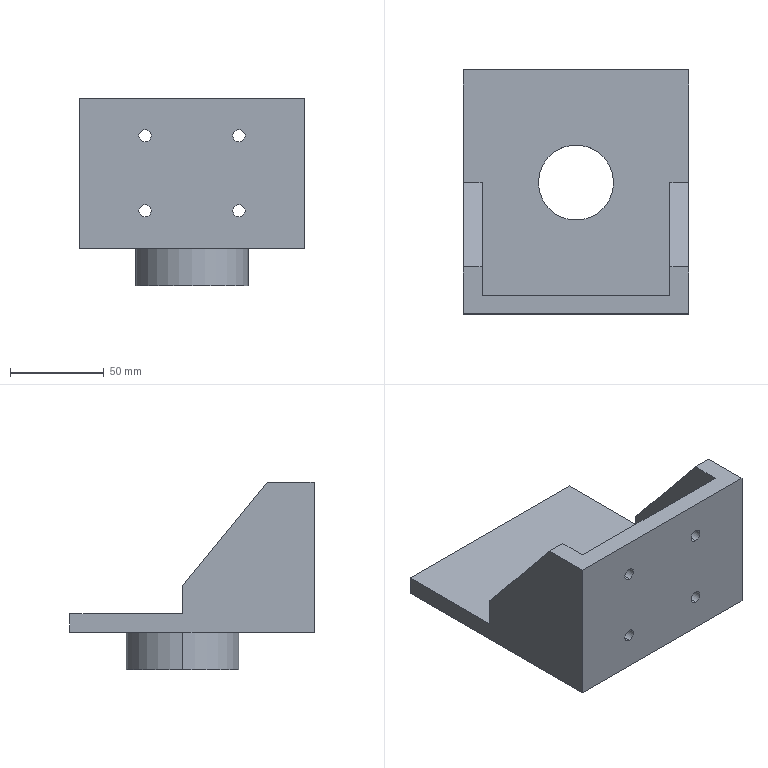Part | NX | features BREP 1 | 1 solid | 30 faces | box 120 x 130 x 100 mm | volume 299431 mm3 | plane 16 | cylinder 14 | commonest cylinder face diameters 6.5 x8 40 x2 52 x2 60 x2
STEP:
#1=CARTESIAN_POINT('',(-30.,0.,20.));
#2=VERTEX_POINT('',#1);
#3=CARTESIAN_POINT('',(30.,0.,20.));
#4=VERTEX_POINT('',#3);
#5=CARTESIAN_POINT('',(0.,0.,20.));
#6=DIRECTION('',(0.,0.,-1.));
#7=DIRECTION('',(-1.,0.,0.));
#8=AXIS2_PLACEMENT_3D('',#5,#6,#7);
#9=CIRCLE('',#8,30.);
#10=EDGE_CURVE('',#2,#4,#9,.T.);
#11=ORIENTED_EDGE('',*,*,#10,.T.);
#12=CARTESIAN_POINT('',(30.,0.,0.));
#13=VERTEX_POINT('',#12);
#14=CARTESIAN_POINT('',(30.,0.,20.));
#15=DIRECTION('',(0.,0.,-1.));
#16=VECTOR('',#15,1000.);
#17=LINE('',#14,#16);
#18=EDGE_CURVE('',#4,#13,#17,.T.);
#19=ORIENTED_EDGE('',*,*,#18,.T.);
#20=CARTESIAN_POINT('',(-30.,0.,0.));
#21=VERTEX_POINT('',#20);
#22=CARTESIAN_POINT('',(0.,0.,0.));
#23=DIRECTION('',(0.,0.,1.));
#24=DIRECTION('',(-1.,0.,0.));
#25=AXIS2_PLACEMENT_3D('',#22,#23,#24);
#26=CIRCLE('',#25,30.);
#27=EDGE_CURVE('',#13,#21,#26,.T.);
#28=ORIENTED_EDGE('',*,*,#27,.T.);
#29=CARTESIAN_POINT('',(-30.,0.,20.));
#30=DIRECTION('',(0.,0.,-1.));
#31=VECTOR('',#30,1000.);
#32=LINE('',#29,#31);
#33=EDGE_CURVE('',#2,#21,#32,.T.);
#34=ORIENTED_EDGE('',*,*,#33,.F.);
#35=EDGE_LOOP('',(#11,#19,#28,#34));
#36=FACE_BOUND('',#35,.T.);
#37=CARTESIAN_POINT('',(0.,0.,20.));
#38=DIRECTION('',(0.,0.,-1.));
#39=DIRECTION('',(-1.,0.,0.));
#40=AXIS2_PLACEMENT_3D('',#37,#38,#39);
#41=CYLINDRICAL_SURFACE('',#40,30.);
#42=ADVANCED_FACE('',(#36),#41,.T.);
#43=CARTESIAN_POINT('',(-25.,-60.,83.25));
#44=VERTEX_POINT('',#43);
#45=CARTESIAN_POINT('',(-25.,-60.,76.75));
#46=VERTEX_POINT('',#45);
#47=CARTESIAN_POINT('',(-25.,-60.,80.));
#48=DIRECTION('',(0.,-1.,0.));
#49=DIRECTION('',(0.,0.,-1.));
#50=AXIS2_PLACEMENT_3D('',#47,#48,#49);
#51=CIRCLE('',#50,3.25);
#52=EDGE_CURVE('',#44,#46,#51,.T.);
#53=ORIENTED_EDGE('',*,*,#52,.F.);
#54=CARTESIAN_POINT('',(-25.,-70.,83.25));
#55=VERTEX_POINT('',#54);
#56=CARTESIAN_POINT('',(-25.,-60.,83.25));
#57=DIRECTION('',(0.,-1.,0.));
#58=VECTOR('',#57,1000.);
#59=LINE('',#56,#58);
#60=EDGE_CURVE('',#44,#55,#59,.T.);
#61=ORIENTED_EDGE('',*,*,#60,.T.);
#62=CARTESIAN_POINT('',(-25.,-70.,76.75));
#63=VERTEX_POINT('',#62);
#64=CARTESIAN_POINT('',(-25.,-70.,80.));
#65=DIRECTION('',(0.,1.,0.));
#66=DIRECTION('',(0.,0.,-1.));
#67=AXIS2_PLACEMENT_3D('',#64,#65,#66);
#68=CIRCLE('',#67,3.25);
#69=EDGE_CURVE('',#63,#55,#68,.T.);
#70=ORIENTED_EDGE('',*,*,#69,.F.);
#71=CARTESIAN_POINT('',(-25.,-60.,76.75));
#72=DIRECTION('',(0.,-1.,0.));
#73=VECTOR('',#72,1000.);
#74=LINE('',#71,#73);
#75=EDGE_CURVE('',#46,#63,#74,.T.);
#76=ORIENTED_EDGE('',*,*,#75,.F.);
#77=EDGE_LOOP('',(#53,#61,#70,#76));
#78=FACE_BOUND('',#77,.T.);
#79=CARTESIAN_POINT('',(-25.,-60.,80.));
#80=DIRECTION('',(0.,-1.,0.));
#81=DIRECTION('',(0.,0.,-1.));
#82=AXIS2_PLACEMENT_3D('',#79,#80,#81);
#83=CYLINDRICAL_SURFACE('',#82,3.25);
#84=ADVANCED_FACE('',(#78),#83,.F.);
#85=CARTESIAN_POINT('',(25.,-60.,83.25));
#86=VERTEX_POINT('',#85);
#87=CARTESIAN_POINT('',(25.,-60.,76.75));
#88=VERTEX_POINT('',#87);
#89=CARTESIAN_POINT('',(25.,-60.,80.));
#90=DIRECTION('',(0.,-1.,0.));
#91=DIRECTION('',(0.,0.,-1.));
#92=AXIS2_PLACEMENT_3D('',#89,#90,#91);
#93=CIRCLE('',#92,3.25);
#94=EDGE_CURVE('',#86,#88,#93,.T.);
#95=ORIENTED_EDGE('',*,*,#94,.F.);
#96=CARTESIAN_POINT('',(25.,-70.,83.25));
#97=VERTEX_POINT('',#96);
#98=CARTESIAN_POINT('',(25.,-60.,83.25));
#99=DIRECTION('',(0.,-1.,0.));
#100=VECTOR('',#99,1000.);
#101=LINE('',#98,#100);
#102=EDGE_CURVE('',#86,#97,#101,.T.);
#103=ORIENTED_EDGE('',*,*,#102,.T.);
#104=CARTESIAN_POINT('',(25.,-70.,76.75));
#105=VERTEX_POINT('',#104);
#106=CARTESIAN_POINT('',(25.,-70.,80.));
#107=DIRECTION('',(0.,1.,0.));
#108=DIRECTION('',(0.,0.,-1.));
#109=AXIS2_PLACEMENT_3D('',#106,#107,#108);
#110=CIRCLE('',#109,3.25);
#111=EDGE_CURVE('',#105,#97,#110,.T.);
#112=ORIENTED_EDGE('',*,*,#111,.F.);
#113=CARTESIAN_POINT('',(25.,-60.,76.75));
#114=DIRECTION('',(0.,-1.,0.));
#115=VECTOR('',#114,1000.);
#116=LINE('',#113,#115);
#117=EDGE_CURVE('',#88,#105,#116,.T.);
#118=ORIENTED_EDGE('',*,*,#117,.F.);
#119=EDGE_LOOP('',(#95,#103,#112,#118));
#120=FACE_BOUND('',#119,.T.);
#121=CARTESIAN_POINT('',(25.,-60.,80.));
#122=DIRECTION('',(0.,-1.,0.));
#123=DIRECTION('',(0.,0.,-1.));
#124=AXIS2_PLACEMENT_3D('',#121,#122,#123);
#125=CYLINDRICAL_SURFACE('',#124,3.25);
#126=ADVANCED_FACE('',(#120),#125,.F.);
#127=CARTESIAN_POINT('',(25.,-60.,43.25));
#128=VERTEX_POINT('',#127);
#129=CARTESIAN_POINT('',(25.,-60.,36.75));
#130=VERTEX_POINT('',#129);
#131=CARTESIAN_POINT('',(25.,-60.,40.));
#132=DIRECTION('',(0.,-1.,0.));
#133=DIRECTION('',(0.,0.,-1.));
#134=AXIS2_PLACEMENT_3D('',#131,#132,#133);
#135=CIRCLE('',#134,3.25);
#136=EDGE_CURVE('',#128,#130,#135,.T.);
#137=ORIENTED_EDGE('',*,*,#136,.F.);
#138=CARTESIAN_POINT('',(25.,-70.,43.25));
#139=VERTEX_POINT('',#138);
#140=CARTESIAN_POINT('',(25.,-60.,43.25));
#141=DIRECTION('',(0.,-1.,0.));
#142=VECTOR('',#141,1000.);
#143=LINE('',#140,#142);
#144=EDGE_CURVE('',#128,#139,#143,.T.);
#145=ORIENTED_EDGE('',*,*,#144,.T.);
#146=CARTESIAN_POINT('',(25.,-70.,36.75));
#147=VERTEX_POINT('',#146);
#148=CARTESIAN_POINT('',(25.,-70.,40.));
#149=DIRECTION('',(0.,1.,0.));
#150=DIRECTION('',(0.,0.,-1.));
#151=AXIS2_PLACEMENT_3D('',#148,#149,#150);
#152=CIRCLE('',#151,3.25);
#153=EDGE_CURVE('',#147,#139,#152,.T.);
#154=ORIENTED_EDGE('',*,*,#153,.F.);
#155=CARTESIAN_POINT('',(25.,-60.,36.75));
#156=DIRECTION('',(0.,-1.,0.));
#157=VECTOR('',#156,1000.);
#158=LINE('',#155,#157);
#159=EDGE_CURVE('',#130,#147,#158,.T.);
#160=ORIENTED_EDGE('',*,*,#159,.F.);
#161=EDGE_LOOP('',(#137,#145,#154,#160));
#162=FACE_BOUND('',#161,.T.);
#163=CARTESIAN_POINT('',(25.,-60.,40.));
#164=DIRECTION('',(0.,-1.,0.));
#165=DIRECTION('',(0.,0.,-1.));
#166=AXIS2_PLACEMENT_3D('',#163,#164,#165);
#167=CYLINDRICAL_SURFACE('',#166,3.25);
#168=ADVANCED_FACE('',(#162),#167,.F.);
#169=CARTESIAN_POINT('',(-25.,-60.,43.25));
#170=VERTEX_POINT('',#169);
#171=CARTESIAN_POINT('',(-25.,-60.,36.75));
#172=VERTEX_POINT('',#171);
#173=CARTESIAN_POINT('',(-25.,-60.,40.));
#174=DIRECTION('',(0.,-1.,0.));
#175=DIRECTION('',(0.,0.,-1.));
#176=AXIS2_PLACEMENT_3D('',#173,#174,#175);
#177=CIRCLE('',#176,3.25);
#178=EDGE_CURVE('',#170,#172,#177,.T.);
#179=ORIENTED_EDGE('',*,*,#178,.F.);
#180=CARTESIAN_POINT('',(-25.,-70.,43.25));
#181=VERTEX_POINT('',#180);
#182=CARTESIAN_POINT('',(-25.,-60.,43.25));
#183=DIRECTION('',(0.,-1.,0.));
#184=VECTOR('',#183,1000.);
#185=LINE('',#182,#184);
#186=EDGE_CURVE('',#170,#181,#185,.T.);
#187=ORIENTED_EDGE('',*,*,#186,.T.);
#188=CARTESIAN_POINT('',(-25.,-70.,36.75));
#189=VERTEX_POINT('',#188);
#190=CARTESIAN_POINT('',(-25.,-70.,40.));
#191=DIRECTION('',(0.,1.,0.));
#192=DIRECTION('',(0.,0.,-1.));
#193=AXIS2_PLACEMENT_3D('',#190,#191,#192);
#194=CIRCLE('',#193,3.25);
#195=EDGE_CURVE('',#189,#181,#194,.T.);
#196=ORIENTED_EDGE('',*,*,#195,.F.);
#197=CARTESIAN_POINT('',(-25.,-60.,36.75));
#198=DIRECTION('',(0.,-1.,0.));
#199=VECTOR('',#198,1000.);
#200=LINE('',#197,#199);
#201=EDGE_CURVE('',#172,#189,#200,.T.);
#202=ORIENTED_EDGE('',*,*,#201,.F.);
#203=EDGE_LOOP('',(#179,#187,#196,#202));
#204=FACE_BOUND('',#203,.T.);
#205=CARTESIAN_POINT('',(-25.,-60.,40.));
#206=DIRECTION('',(0.,-1.,0.));
#207=DIRECTION('',(0.,0.,-1.));
#208=AXIS2_PLACEMENT_3D('',#205,#206,#207);
#209=CYLINDRICAL_SURFACE('',#208,3.25);
#210=ADVANCED_FACE('',(#204),#209,.F.);
#211=CARTESIAN_POINT('',(26.,0.,20.));
#212=VERTEX_POINT('',#211);
#213=CARTESIAN_POINT('',(-26.,0.,20.));
#214=VERTEX_POINT('',#213);
#215=CARTESIAN_POINT('',(0.,0.,20.));
#216=DIRECTION('',(0.,0.,-1.));
#217=DIRECTION('',(-1.,0.,0.));
#218=AXIS2_PLACEMENT_3D('',#215,#216,#217);
#219=CIRCLE('',#218,26.);
#220=EDGE_CURVE('',#212,#214,#219,.T.);
#221=ORIENTED_EDGE('',*,*,#220,.F.);
#222=CARTESIAN_POINT('',(26.,0.,0.));
#223=VERTEX_POINT('',#222);
#224=CARTESIAN_POINT('',(26.,0.,20.));
#225=DIRECTION('',(0.,0.,-1.));
#226=VECTOR('',#225,1000.);
#227=LINE('',#224,#226);
#228=EDGE_CURVE('',#212,#223,#227,.T.);
#229=ORIENTED_EDGE('',*,*,#228,.T.);
#230=CARTESIAN_POINT('',(-26.,0.,0.));
#231=VERTEX_POINT('',#230);
#232=CARTESIAN_POINT('',(0.,0.,0.));
#233=DIRECTION('',(0.,0.,-1.));
#234=DIRECTION('',(-1.,0.,0.));
#235=AXIS2_PLACEMENT_3D('',#232,#233,#234);
#236=CIRCLE('',#235,26.);
#237=EDGE_CURVE('',#223,#231,#236,.T.);
#238=ORIENTED_EDGE('',*,*,#237,.T.);
#239=CARTESIAN_POINT('',(-26.,0.,20.));
#240=DIRECTION('',(0.,0.,-1.));
#241=VECTOR('',#240,1000.);
#242=LINE('',#239,#241);
#243=EDGE_CURVE('',#214,#231,#242,.T.);
#244=ORIENTED_EDGE('',*,*,#243,.F.);
#245=EDGE_LOOP('',(#221,#229,#238,#244));
#246=FACE_BOUND('',#245,.T.);
#247=CARTESIAN_POINT('',(0.,0.,20.));
#248=DIRECTION('',(0.,0.,-1.));
#249=DIRECTION('',(-1.,0.,0.));
#250=AXIS2_PLACEMENT_3D('',#247,#248,#249);
#251=CYLINDRICAL_SURFACE('',#250,26.);
#252=ADVANCED_FACE('',(#246),#251,.F.);
#253=CARTESIAN_POINT('',(20.,0.,30.));
#254=VERTEX_POINT('',#253);
#255=CARTESIAN_POINT('',(-20.,0.,30.));
#256=VERTEX_POINT('',#255);
#257=CARTESIAN_POINT('',(0.,0.,30.));
#258=DIRECTION('',(0.,0.,-1.));
#259=DIRECTION('',(-1.,0.,0.));
#260=AXIS2_PLACEMENT_3D('',#257,#258,#259);
#261=CIRCLE('',#260,20.);
#262=EDGE_CURVE('',#254,#256,#261,.T.);
#263=ORIENTED_EDGE('',*,*,#262,.F.);
#264=CARTESIAN_POINT('',(20.,0.,20.));
#265=VERTEX_POINT('',#264);
#266=CARTESIAN_POINT('',(20.,0.,30.));
#267=DIRECTION('',(0.,0.,-1.));
#268=VECTOR('',#267,1000.);
#269=LINE('',#266,#268);
#270=EDGE_CURVE('',#254,#265,#269,.T.);
#271=ORIENTED_EDGE('',*,*,#270,.T.);
#272=CARTESIAN_POINT('',(-20.,0.,20.));
#273=VERTEX_POINT('',#272);
#274=CARTESIAN_POINT('',(0.,0.,20.));
#275=DIRECTION('',(0.,0.,1.));
#276=DIRECTION('',(-1.,0.,0.));
#277=AXIS2_PLACEMENT_3D('',#274,#275,#276);
#278=CIRCLE('',#277,20.);
#279=EDGE_CURVE('',#273,#265,#278,.T.);
#280=ORIENTED_EDGE('',*,*,#279,.F.);
#281=CARTESIAN_POINT('',(-20.,0.,30.));
#282=DIRECTION('',(0.,0.,-1.));
#283=VECTOR('',#282,1000.);
#284=LINE('',#281,#283);
#285=EDGE_CURVE('',#256,#273,#284,.T.);
#286=ORIENTED_EDGE('',*,*,#285,.F.);
#287=EDGE_LOOP('',(#263,#271,#280,#286));
#288=FACE_BOUND('',#287,.T.);
#289=CARTESIAN_POINT('',(0.,0.,30.));
#290=DIRECTION('',(0.,0.,-1.));
#291=DIRECTION('',(-1.,0.,0.));
#292=AXIS2_PLACEMENT_3D('',#289,#290,#291);
#293=CYLINDRICAL_SURFACE('',#292,20.);
#294=ADVANCED_FACE('',(#288),#293,.F.);
#295=CARTESIAN_POINT('',(-60.,-70.,20.));
#296=VERTEX_POINT('',#295);
#297=CARTESIAN_POINT('',(60.,-70.,20.));
#298=VERTEX_POINT('',#297);
#299=CARTESIAN_POINT('',(60.,-70.,20.));
#300=DIRECTION('',(1.,0.,0.));
#301=VECTOR('',#300,1000.);
#302=LINE('',#299,#301);
#303=EDGE_CURVE('',#296,#298,#302,.T.);
#304=ORIENTED_EDGE('',*,*,#303,.F.);
#305=CARTESIAN_POINT('',(-60.,60.,20.));
#306=VERTEX_POINT('',#305);
#307=CARTESIAN_POINT('',(-60.,-60.,20.));
#308=DIRECTION('',(0.,-1.,0.));
#309=VECTOR('',#308,1000.);
#310=LINE('',#307,#309);
#311=EDGE_CURVE('',#306,#296,#310,.T.);
#312=ORIENTED_EDGE('',*,*,#311,.F.);
#313=CARTESIAN_POINT('',(60.,60.,20.));
#314=VERTEX_POINT('',#313);
#315=CARTESIAN_POINT('',(60.,60.,20.));
#316=DIRECTION('',(-1.,0.,0.));
#317=VECTOR('',#316,1000.);
#318=LINE('',#315,#317);
#319=EDGE_CURVE('',#314,#306,#318,.T.);
#320=ORIENTED_EDGE('',*,*,#319,.F.);
#321=CARTESIAN_POINT('',(60.,-60.,20.));
#322=DIRECTION('',(0.,1.,0.));
#323=VECTOR('',#322,1000.);
#324=LINE('',#321,#323);
#325=EDGE_CURVE('',#298,#314,#324,.T.);
#326=ORIENTED_EDGE('',*,*,#325,.F.);
#327=EDGE_LOOP('',(#304,#312,#320,#326));
#328=FACE_BOUND('',#327,.T.);
#329=ORIENTED_EDGE('',*,*,#10,.F.);
#330=CARTESIAN_POINT('',(0.,0.,20.));
#331=DIRECTION('',(0.,0.,-1.));
#332=DIRECTION('',(-1.,0.,0.));
#333=AXIS2_PLACEMENT_3D('',#330,#331,#332);
#334=CIRCLE('',#333,30.);
#335=EDGE_CURVE('',#4,#2,#334,.T.);
#336=ORIENTED_EDGE('',*,*,#335,.F.);
#337=EDGE_LOOP('',(#329,#336));
#338=FACE_BOUND('',#337,.T.);
#339=CARTESIAN_POINT('',(60.,-60.,20.));
#340=DIRECTION('',(0.,0.,1.));
#341=DIRECTION('',(1.,0.,0.));
#342=AXIS2_PLACEMENT_3D('',#339,#340,#341);
#343=PLANE('',#342);
#344=ADVANCED_FACE('',(#328,#338),#343,.F.);
#345=ORIENTED_EDGE('',*,*,#18,.F.);
#346=ORIENTED_EDGE('',*,*,#335,.T.);
#347=ORIENTED_EDGE('',*,*,#33,.T.);
#348=CARTESIAN_POINT('',(0.,0.,0.));
#349=DIRECTION('',(0.,0.,1.));
#350=DIRECTION('',(-1.,0.,0.));
#351=AXIS2_PLACEMENT_3D('',#348,#349,#350);
#352=CIRCLE('',#351,30.);
#353=EDGE_CURVE('',#21,#13,#352,.T.);
#354=ORIENTED_EDGE('',*,*,#353,.T.);
#355=EDGE_LOOP('',(#345,#346,#347,#354));
#356=FACE_BOUND('',#355,.T.);
#357=CARTESIAN_POINT('',(0.,0.,20.));
#358=DIRECTION('',(0.,0.,-1.));
#359=DIRECTION('',(-1.,0.,0.));
#360=AXIS2_PLACEMENT_3D('',#357,#358,#359);
#361=CYLINDRICAL_SURFACE('',#360,30.);
#362=ADVANCED_FACE('',(#356),#361,.T.);
#363=CARTESIAN_POINT('',(60.,0.,45.));
#364=VERTEX_POINT('',#363);
#365=CARTESIAN_POINT('',(60.,0.,30.));
#366=VERTEX_POINT('',#365);
#367=CARTESIAN_POINT('',(60.,0.,30.));
#368=DIRECTION('',(0.,0.,-1.));
#369=VECTOR('',#368,1000.);
#370=LINE('',#367,#369);
#371=EDGE_CURVE('',#364,#366,#370,.T.);
#372=ORIENTED_EDGE('',*,*,#371,.F.);
#373=CARTESIAN_POINT('',(60.,-45.,100.));
#374=VERTEX_POINT('',#373);
#375=CARTESIAN_POINT('',(60.,-45.,100.));
#376=DIRECTION('',(0.,0.6332,-0.774));
#377=VECTOR('',#376,1000.);
#378=LINE('',#375,#377);
#379=EDGE_CURVE('',#374,#364,#378,.T.);
#380=ORIENTED_EDGE('',*,*,#379,.F.);
#381=CARTESIAN_POINT('',(60.,-70.,100.));
#382=VERTEX_POINT('',#381);
#383=CARTESIAN_POINT('',(60.,60.,100.));
#384=DIRECTION('',(0.,1.,0.));
#385=VECTOR('',#384,1000.);
#386=LINE('',#383,#385);
#387=EDGE_CURVE('',#382,#374,#386,.T.);
#388=ORIENTED_EDGE('',*,*,#387,.F.);
#389=CARTESIAN_POINT('',(60.,-70.,30.));
#390=DIRECTION('',(0.,0.,1.));
#391=VECTOR('',#390,1000.);
#392=LINE('',#389,#391);
#393=EDGE_CURVE('',#298,#382,#392,.T.);
#394=ORIENTED_EDGE('',*,*,#393,.F.);
#395=ORIENTED_EDGE('',*,*,#325,.T.);
#396=CARTESIAN_POINT('',(60.,60.,30.));
#397=VERTEX_POINT('',#396);
#398=CARTESIAN_POINT('',(60.,60.,30.));
#399=DIRECTION('',(0.,0.,-1.));
#400=VECTOR('',#399,1000.);
#401=LINE('',#398,#400);
#402=EDGE_CURVE('',#397,#314,#401,.T.);
#403=ORIENTED_EDGE('',*,*,#402,.F.);
#404=CARTESIAN_POINT('',(60.,60.,30.));
#405=DIRECTION('',(0.,1.,0.));
#406=VECTOR('',#405,1000.);
#407=LINE('',#404,#406);
#408=EDGE_CURVE('',#366,#397,#407,.T.);
#409=ORIENTED_EDGE('',*,*,#408,.F.);
#410=EDGE_LOOP('',(#372,#380,#388,#394,#395,#403,#409));
#411=FACE_BOUND('',#410,.T.);
#412=CARTESIAN_POINT('',(60.,60.,30.));
#413=DIRECTION('',(-1.,0.,0.));
#414=DIRECTION('',(0.,1.,0.));
#415=AXIS2_PLACEMENT_3D('',#412,#413,#414);
#416=PLANE('',#415);
#417=ADVANCED_FACE('',(#411),#416,.F.);
#418=ORIENTED_EDGE('',*,*,#393,.T.);
#419=CARTESIAN_POINT('',(-60.,-70.,100.));
#420=VERTEX_POINT('',#419);
#421=CARTESIAN_POINT('',(-140.623,-70.,100.));
#422=DIRECTION('',(-1.,0.,0.));
#423=VECTOR('',#422,1000.);
#424=LINE('',#421,#423);
#425=EDGE_CURVE('',#382,#420,#424,.T.);
#426=ORIENTED_EDGE('',*,*,#425,.T.);
#427=CARTESIAN_POINT('',(-60.,-70.,100.));
#428=DIRECTION('',(0.,0.,-1.));
#429=VECTOR('',#428,1000.);
#430=LINE('',#427,#429);
#431=EDGE_CURVE('',#420,#296,#430,.T.);
#432=ORIENTED_EDGE('',*,*,#431,.T.);
#433=ORIENTED_EDGE('',*,*,#303,.T.);
#434=EDGE_LOOP('',(#418,#426,#432,#433));
#435=FACE_BOUND('',#434,.T.);
#436=ORIENTED_EDGE('',*,*,#69,.T.);
#437=CARTESIAN_POINT('',(-25.,-70.,80.));
#438=DIRECTION('',(0.,1.,0.));
#439=DIRECTION('',(0.,0.,-1.));
#440=AXIS2_PLACEMENT_3D('',#437,#438,#439);
#441=CIRCLE('',#440,3.25);
#442=EDGE_CURVE('',#55,#63,#441,.T.);
#443=ORIENTED_EDGE('',*,*,#442,.T.);
#444=EDGE_LOOP('',(#436,#443));
#445=FACE_BOUND('',#444,.T.);
#446=ORIENTED_EDGE('',*,*,#111,.T.);
#447=CARTESIAN_POINT('',(25.,-70.,80.));
#448=DIRECTION('',(0.,1.,0.));
#449=DIRECTION('',(0.,0.,-1.));
#450=AXIS2_PLACEMENT_3D('',#447,#448,#449);
#451=CIRCLE('',#450,3.25);
#452=EDGE_CURVE('',#97,#105,#451,.T.);
#453=ORIENTED_EDGE('',*,*,#452,.T.);
#454=EDGE_LOOP('',(#446,#453));
#455=FACE_BOUND('',#454,.T.);
#456=ORIENTED_EDGE('',*,*,#153,.T.);
#457=CARTESIAN_POINT('',(25.,-70.,40.));
#458=DIRECTION('',(0.,1.,0.));
#459=DIRECTION('',(0.,0.,-1.));
#460=AXIS2_PLACEMENT_3D('',#457,#458,#459);
#461=CIRCLE('',#460,3.25);
#462=EDGE_CURVE('',#139,#147,#461,.T.);
#463=ORIENTED_EDGE('',*,*,#462,.T.);
#464=EDGE_LOOP('',(#456,#463));
#465=FACE_BOUND('',#464,.T.);
#466=ORIENTED_EDGE('',*,*,#195,.T.);
#467=CARTESIAN_POINT('',(-25.,-70.,40.));
#468=DIRECTION('',(0.,1.,0.));
#469=DIRECTION('',(0.,0.,-1.));
#470=AXIS2_PLACEMENT_3D('',#467,#468,#469);
#471=CIRCLE('',#470,3.25);
#472=EDGE_CURVE('',#181,#189,#471,.T.);
#473=ORIENTED_EDGE('',*,*,#472,.T.);
#474=EDGE_LOOP('',(#466,#473));
#475=FACE_BOUND('',#474,.T.);
#476=CARTESIAN_POINT('',(-140.623,-70.,100.));
#477=DIRECTION('',(0.,-1.,0.));
#478=DIRECTION('',(0.,0.,-1.));
#479=AXIS2_PLACEMENT_3D('',#476,#477,#478);
#480=PLANE('',#479);
#481=ADVANCED_FACE('',(#435,#445,#455,#465,#475),#480,.T.);
#482=CARTESIAN_POINT('',(-60.,60.,30.));
#483=VERTEX_POINT('',#482);
#484=CARTESIAN_POINT('',(-60.,0.,30.));
#485=VERTEX_POINT('',#484);
#486=CARTESIAN_POINT('',(-60.,60.,30.));
#487=DIRECTION('',(0.,-1.,0.));
#488=VECTOR('',#487,1000.);
#489=LINE('',#486,#488);
#490=EDGE_CURVE('',#483,#485,#489,.T.);
#491=ORIENTED_EDGE('',*,*,#490,.F.);
#492=CARTESIAN_POINT('',(-60.,60.,30.));
#493=DIRECTION('',(0.,0.,1.));
#494=VECTOR('',#493,1000.);
#495=LINE('',#492,#494);
#496=EDGE_CURVE('',#306,#483,#495,.T.);
#497=ORIENTED_EDGE('',*,*,#496,.F.);
#498=ORIENTED_EDGE('',*,*,#311,.T.);
#499=ORIENTED_EDGE('',*,*,#431,.F.);
#500=CARTESIAN_POINT('',(-60.,-45.,100.));
#501=VERTEX_POINT('',#500);
#502=CARTESIAN_POINT('',(-60.,60.,100.));
#503=DIRECTION('',(0.,-1.,0.));
#504=VECTOR('',#503,1000.);
#505=LINE('',#502,#504);
#506=EDGE_CURVE('',#501,#420,#505,.T.);
#507=ORIENTED_EDGE('',*,*,#506,.F.);
#508=CARTESIAN_POINT('',(-60.,0.,45.));
#509=VERTEX_POINT('',#508);
#510=CARTESIAN_POINT('',(-60.,0.,45.));
#511=DIRECTION('',(0.,-0.6332,0.774));
#512=VECTOR('',#511,1000.);
#513=LINE('',#510,#512);
#514=EDGE_CURVE('',#509,#501,#513,.T.);
#515=ORIENTED_EDGE('',*,*,#514,.F.);
#516=CARTESIAN_POINT('',(-60.,0.,30.));
#517=DIRECTION('',(0.,0.,1.));
#518=VECTOR('',#517,1000.);
#519=LINE('',#516,#518);
#520=EDGE_CURVE('',#485,#509,#519,.T.);
#521=ORIENTED_EDGE('',*,*,#520,.F.);
#522=EDGE_LOOP('',(#491,#497,#498,#499,#507,#515,#521));
#523=FACE_BOUND('',#522,.T.);
#524=CARTESIAN_POINT('',(-60.,60.,30.));
#525=DIRECTION('',(1.,0.,0.));
#526=DIRECTION('',(0.,1.,0.));
#527=AXIS2_PLACEMENT_3D('',#524,#525,#526);
#528=PLANE('',#527);
#529=ADVANCED_FACE('',(#523),#528,.F.);
#530=ORIENTED_EDGE('',*,*,#496,.T.);
#531=CARTESIAN_POINT('',(-60.,60.,30.));
#532=DIRECTION('',(-1.,0.,0.));
#533=VECTOR('',#532,1000.);
#534=LINE('',#531,#533);
#535=EDGE_CURVE('',#397,#483,#534,.T.);
#536=ORIENTED_EDGE('',*,*,#535,.F.);
#537=ORIENTED_EDGE('',*,*,#402,.T.);
#538=ORIENTED_EDGE('',*,*,#319,.T.);
#539=EDGE_LOOP('',(#530,#536,#537,#538));
#540=FACE_BOUND('',#539,.T.);
#541=CARTESIAN_POINT('',(-60.,60.,30.));
#542=DIRECTION('',(0.,-1.,0.));
#543=DIRECTION('',(0.,0.,-1.));
#544=AXIS2_PLACEMENT_3D('',#541,#542,#543);
#545=PLANE('',#544);
#546=ADVANCED_FACE('',(#540),#545,.F.);
#547=ORIENTED_EDGE('',*,*,#353,.F.);
#548=ORIENTED_EDGE('',*,*,#27,.F.);
#549=EDGE_LOOP('',(#547,#548));
#550=FACE_BOUND('',#549,.T.);
#551=CARTESIAN_POINT('',(0.,0.,0.));
#552=DIRECTION('',(0.,0.,-1.));
#553=DIRECTION('',(-1.,0.,0.));
#554=AXIS2_PLACEMENT_3D('',#551,#552,#553);
#555=CIRCLE('',#554,26.);
#556=EDGE_CURVE('',#231,#223,#555,.T.);
#557=ORIENTED_EDGE('',*,*,#556,.F.);
#558=ORIENTED_EDGE('',*,*,#237,.F.);
#559=EDGE_LOOP('',(#557,#558));
#560=FACE_BOUND('',#559,.T.);
#561=CARTESIAN_POINT('',(0.,0.,0.));
#562=DIRECTION('',(0.,0.,1.));
#563=DIRECTION('',(1.,0.,0.));
#564=AXIS2_PLACEMENT_3D('',#561,#562,#563);
#565=PLANE('',#564);
#566=ADVANCED_FACE('',(#550,#560),#565,.F.);
#567=ORIENTED_EDGE('',*,*,#535,.T.);
#568=ORIENTED_EDGE('',*,*,#490,.T.);
#569=CARTESIAN_POINT('',(-50.,0.,30.));
#570=VERTEX_POINT('',#569);
#571=CARTESIAN_POINT('',(60.,0.,30.));
#572=DIRECTION('',(1.,0.,0.));
#573=VECTOR('',#572,1000.);
#574=LINE('',#571,#573);
#575=EDGE_CURVE('',#485,#570,#574,.T.);
#576=ORIENTED_EDGE('',*,*,#575,.T.);
#577=CARTESIAN_POINT('',(-50.,-60.,30.));
#578=VERTEX_POINT('',#577);
#579=CARTESIAN_POINT('',(-50.,-60.,30.));
#580=DIRECTION('',(0.,-1.,0.));
#581=VECTOR('',#580,1000.);
#582=LINE('',#579,#581);
#583=EDGE_CURVE('',#570,#578,#582,.T.);
#584=ORIENTED_EDGE('',*,*,#583,.T.);
#585=CARTESIAN_POINT('',(50.,-60.,30.));
#586=VERTEX_POINT('',#585);
#587=CARTESIAN_POINT('',(60.,-60.,30.));
#588=DIRECTION('',(1.,0.,0.));
#589=VECTOR('',#588,1000.);
#590=LINE('',#587,#589);
#591=EDGE_CURVE('',#578,#586,#590,.T.);
#592=ORIENTED_EDGE('',*,*,#591,.T.);
#593=CARTESIAN_POINT('',(50.,0.,30.));
#594=VERTEX_POINT('',#593);
#595=CARTESIAN_POINT('',(50.,-60.,30.));
#596=DIRECTION('',(0.,1.,0.));
#597=VECTOR('',#596,1000.);
#598=LINE('',#595,#597);
#599=EDGE_CURVE('',#586,#594,#598,.T.);
#600=ORIENTED_EDGE('',*,*,#599,.T.);
#601=CARTESIAN_POINT('',(60.,0.,30.));
#602=DIRECTION('',(1.,0.,0.));
#603=VECTOR('',#602,1000.);
#604=LINE('',#601,#603);
#605=EDGE_CURVE('',#594,#366,#604,.T.);
#606=ORIENTED_EDGE('',*,*,#605,.T.);
#607=ORIENTED_EDGE('',*,*,#408,.T.);
#608=EDGE_LOOP('',(#567,#568,#576,#584,#592,#600,#606,#607));
#609=FACE_BOUND('',#608,.T.);
#610=CARTESIAN_POINT('',(0.,0.,30.));
#611=DIRECTION('',(0.,0.,-1.));
#612=DIRECTION('',(-1.,0.,0.));
#613=AXIS2_PLACEMENT_3D('',#610,#611,#612);
#614=CIRCLE('',#613,20.);
#615=EDGE_CURVE('',#256,#254,#614,.T.);
#616=ORIENTED_EDGE('',*,*,#615,.T.);
#617=ORIENTED_EDGE('',*,*,#262,.T.);
#618=EDGE_LOOP('',(#616,#617));
#619=FACE_BOUND('',#618,.T.);
#620=CARTESIAN_POINT('',(60.,-60.,30.));
#621=DIRECTION('',(0.,0.,1.));
#622=DIRECTION('',(1.,0.,0.));
#623=AXIS2_PLACEMENT_3D('',#620,#621,#622);
#624=PLANE('',#623);
#625=ADVANCED_FACE('',(#609,#619),#624,.T.);
#626=CARTESIAN_POINT('',(50.,0.,45.));
#627=VERTEX_POINT('',#626);
#628=CARTESIAN_POINT('',(50.,0.,45.));
#629=DIRECTION('',(0.,0.,1.));
#630=VECTOR('',#629,1000.);
#631=LINE('',#628,#630);
#632=EDGE_CURVE('',#594,#627,#631,.T.);
#633=ORIENTED_EDGE('',*,*,#632,.T.);
#634=CARTESIAN_POINT('',(50.,0.,45.));
#635=DIRECTION('',(1.,0.,0.));
#636=VECTOR('',#635,1000.);
#637=LINE('',#634,#636);
#638=EDGE_CURVE('',#627,#364,#637,.T.);
#639=ORIENTED_EDGE('',*,*,#638,.T.);
#640=ORIENTED_EDGE('',*,*,#371,.T.);
#641=ORIENTED_EDGE('',*,*,#605,.F.);
#642=EDGE_LOOP('',(#633,#639,#640,#641));
#643=FACE_BOUND('',#642,.T.);
#644=CARTESIAN_POINT('',(50.,0.,45.));
#645=DIRECTION('',(0.,1.,0.));
#646=DIRECTION('',(0.,0.,-1.));
#647=AXIS2_PLACEMENT_3D('',#644,#645,#646);
#648=PLANE('',#647);
#649=ADVANCED_FACE('',(#643),#648,.T.);
#650=CARTESIAN_POINT('',(50.,-45.,100.));
#651=VERTEX_POINT('',#650);
#652=CARTESIAN_POINT('',(50.,-45.,100.));
#653=DIRECTION('',(0.,-0.6332,0.774));
#654=VECTOR('',#653,1000.);
#655=LINE('',#652,#654);
#656=EDGE_CURVE('',#627,#651,#655,.T.);
#657=ORIENTED_EDGE('',*,*,#656,.T.);
#658=CARTESIAN_POINT('',(50.,-45.,100.));
#659=DIRECTION('',(1.,0.,0.));
#660=VECTOR('',#659,1000.);
#661=LINE('',#658,#660);
#662=EDGE_CURVE('',#651,#374,#661,.T.);
#663=ORIENTED_EDGE('',*,*,#662,.T.);
#664=ORIENTED_EDGE('',*,*,#379,.T.);
#665=ORIENTED_EDGE('',*,*,#638,.F.);
#666=EDGE_LOOP('',(#657,#663,#664,#665));
#667=FACE_BOUND('',#666,.T.);
#668=CARTESIAN_POINT('',(50.,-45.,100.));
#669=DIRECTION('',(0.,0.774,0.6332));
#670=DIRECTION('',(1.,0.,0.));
#671=AXIS2_PLACEMENT_3D('',#668,#669,#670);
#672=PLANE('',#671);
#673=ADVANCED_FACE('',(#667),#672,.T.);
#674=CARTESIAN_POINT('',(-50.,-60.,100.));
#675=VERTEX_POINT('',#674);
#676=CARTESIAN_POINT('',(-50.,-45.,100.));
#677=VERTEX_POINT('',#676);
#678=CARTESIAN_POINT('',(-50.,-60.,100.));
#679=DIRECTION('',(0.,1.,0.));
#680=VECTOR('',#679,1000.);
#681=LINE('',#678,#680);
#682=EDGE_CURVE('',#675,#677,#681,.T.);
#683=ORIENTED_EDGE('',*,*,#682,.T.);
#684=CARTESIAN_POINT('',(-140.623,-45.,100.));
#685=DIRECTION('',(-1.,0.,0.));
#686=VECTOR('',#685,1000.);
#687=LINE('',#684,#686);
#688=EDGE_CURVE('',#677,#501,#687,.T.);
#689=ORIENTED_EDGE('',*,*,#688,.T.);
#690=ORIENTED_EDGE('',*,*,#506,.T.);
#691=ORIENTED_EDGE('',*,*,#425,.F.);
#692=ORIENTED_EDGE('',*,*,#387,.T.);
#693=ORIENTED_EDGE('',*,*,#662,.F.);
#694=CARTESIAN_POINT('',(50.,-60.,100.));
#695=VERTEX_POINT('',#694);
#696=CARTESIAN_POINT('',(50.,-60.,100.));
#697=DIRECTION('',(0.,-1.,0.));
#698=VECTOR('',#697,1000.);
#699=LINE('',#696,#698);
#700=EDGE_CURVE('',#651,#695,#699,.T.);
#701=ORIENTED_EDGE('',*,*,#700,.T.);
#702=CARTESIAN_POINT('',(-140.623,-60.,100.));
#703=DIRECTION('',(-1.,0.,0.));
#704=VECTOR('',#703,1000.);
#705=LINE('',#702,#704);
#706=EDGE_CURVE('',#695,#675,#705,.T.);
#707=ORIENTED_EDGE('',*,*,#706,.T.);
#708=EDGE_LOOP('',(#683,#689,#690,#691,#692,#693,#701,#707));
#709=FACE_BOUND('',#708,.T.);
#710=CARTESIAN_POINT('',(-140.623,-60.,100.));
#711=DIRECTION('',(0.,0.,1.));
#712=DIRECTION('',(1.,0.,0.));
#713=AXIS2_PLACEMENT_3D('',#710,#711,#712);
#714=PLANE('',#713);
#715=ADVANCED_FACE('',(#709),#714,.T.);
#716=ORIENTED_EDGE('',*,*,#60,.F.);
#717=CARTESIAN_POINT('',(-25.,-60.,80.));
#718=DIRECTION('',(0.,-1.,0.));
#719=DIRECTION('',(0.,0.,-1.));
#720=AXIS2_PLACEMENT_3D('',#717,#718,#719);
#721=CIRCLE('',#720,3.25);
#722=EDGE_CURVE('',#46,#44,#721,.T.);
#723=ORIENTED_EDGE('',*,*,#722,.F.);
#724=ORIENTED_EDGE('',*,*,#75,.T.);
#725=ORIENTED_EDGE('',*,*,#442,.F.);
#726=EDGE_LOOP('',(#716,#723,#724,#725));
#727=FACE_BOUND('',#726,.T.);
#728=CARTESIAN_POINT('',(-25.,-60.,80.));
#729=DIRECTION('',(0.,-1.,0.));
#730=DIRECTION('',(0.,0.,-1.));
#731=AXIS2_PLACEMENT_3D('',#728,#729,#730);
#732=CYLINDRICAL_SURFACE('',#731,3.25);
#733=ADVANCED_FACE('',(#727),#732,.F.);
#734=ORIENTED_EDGE('',*,*,#102,.F.);
#735=CARTESIAN_POINT('',(25.,-60.,80.));
#736=DIRECTION('',(0.,-1.,0.));
#737=DIRECTION('',(0.,0.,-1.));
#738=AXIS2_PLACEMENT_3D('',#735,#736,#737);
#739=CIRCLE('',#738,3.25);
#740=EDGE_CURVE('',#88,#86,#739,.T.);
#741=ORIENTED_EDGE('',*,*,#740,.F.);
#742=ORIENTED_EDGE('',*,*,#117,.T.);
#743=ORIENTED_EDGE('',*,*,#452,.F.);
#744=EDGE_LOOP('',(#734,#741,#742,#743));
#745=FACE_BOUND('',#744,.T.);
#746=CARTESIAN_POINT('',(25.,-60.,80.));
#747=DIRECTION('',(0.,-1.,0.));
#748=DIRECTION('',(0.,0.,-1.));
#749=AXIS2_PLACEMENT_3D('',#746,#747,#748);
#750=CYLINDRICAL_SURFACE('',#749,3.25);
#751=ADVANCED_FACE('',(#745),#750,.F.);
#752=ORIENTED_EDGE('',*,*,#144,.F.);
#753=CARTESIAN_POINT('',(25.,-60.,40.));
#754=DIRECTION('',(0.,-1.,0.));
#755=DIRECTION('',(0.,0.,-1.));
#756=AXIS2_PLACEMENT_3D('',#753,#754,#755);
#757=CIRCLE('',#756,3.25);
#758=EDGE_CURVE('',#130,#128,#757,.T.);
#759=ORIENTED_EDGE('',*,*,#758,.F.);
#760=ORIENTED_EDGE('',*,*,#159,.T.);
#761=ORIENTED_EDGE('',*,*,#462,.F.);
#762=EDGE_LOOP('',(#752,#759,#760,#761));
#763=FACE_BOUND('',#762,.T.);
#764=CARTESIAN_POINT('',(25.,-60.,40.));
#765=DIRECTION('',(0.,-1.,0.));
#766=DIRECTION('',(0.,0.,-1.));
#767=AXIS2_PLACEMENT_3D('',#764,#765,#766);
#768=CYLINDRICAL_SURFACE('',#767,3.25);
#769=ADVANCED_FACE('',(#763),#768,.F.);
#770=ORIENTED_EDGE('',*,*,#186,.F.);
#771=CARTESIAN_POINT('',(-25.,-60.,40.));
#772=DIRECTION('',(0.,-1.,0.));
#773=DIRECTION('',(0.,0.,-1.));
#774=AXIS2_PLACEMENT_3D('',#771,#772,#773);
#775=CIRCLE('',#774,3.25);
#776=EDGE_CURVE('',#172,#170,#775,.T.);
#777=ORIENTED_EDGE('',*,*,#776,.F.);
#778=ORIENTED_EDGE('',*,*,#201,.T.);
#779=ORIENTED_EDGE('',*,*,#472,.F.);
#780=EDGE_LOOP('',(#770,#777,#778,#779));
#781=FACE_BOUND('',#780,.T.);
#782=CARTESIAN_POINT('',(-25.,-60.,40.));
#783=DIRECTION('',(0.,-1.,0.));
#784=DIRECTION('',(0.,0.,-1.));
#785=AXIS2_PLACEMENT_3D('',#782,#783,#784);
#786=CYLINDRICAL_SURFACE('',#785,3.25);
#787=ADVANCED_FACE('',(#781),#786,.F.);
#788=ORIENTED_EDGE('',*,*,#520,.T.);
#789=CARTESIAN_POINT('',(-50.,0.,45.));
#790=VERTEX_POINT('',#789);
#791=CARTESIAN_POINT('',(-60.,0.,45.));
#792=DIRECTION('',(1.,0.,0.));
#793=VECTOR('',#792,1000.);
#794=LINE('',#791,#793);
#795=EDGE_CURVE('',#509,#790,#794,.T.);
#796=ORIENTED_EDGE('',*,*,#795,.T.);
#797=CARTESIAN_POINT('',(-50.,0.,45.));
#798=DIRECTION('',(0.,0.,-1.));
#799=VECTOR('',#798,1000.);
#800=LINE('',#797,#799);
#801=EDGE_CURVE('',#790,#570,#800,.T.);
#802=ORIENTED_EDGE('',*,*,#801,.T.);
#803=ORIENTED_EDGE('',*,*,#575,.F.);
#804=EDGE_LOOP('',(#788,#796,#802,#803));
#805=FACE_BOUND('',#804,.T.);
#806=CARTESIAN_POINT('',(-60.,0.,45.));
#807=DIRECTION('',(0.,1.,0.));
#808=DIRECTION('',(0.,0.,-1.));
#809=AXIS2_PLACEMENT_3D('',#806,#807,#808);
#810=PLANE('',#809);
#811=ADVANCED_FACE('',(#805),#810,.T.);
#812=ORIENTED_EDGE('',*,*,#514,.T.);
#813=ORIENTED_EDGE('',*,*,#688,.F.);
#814=CARTESIAN_POINT('',(-50.,-45.,100.));
#815=DIRECTION('',(0.,0.6332,-0.774));
#816=VECTOR('',#815,1000.);
#817=LINE('',#814,#816);
#818=EDGE_CURVE('',#677,#790,#817,.T.);
#819=ORIENTED_EDGE('',*,*,#818,.T.);
#820=ORIENTED_EDGE('',*,*,#795,.F.);
#821=EDGE_LOOP('',(#812,#813,#819,#820));
#822=FACE_BOUND('',#821,.T.);
#823=CARTESIAN_POINT('',(-60.,-45.,100.));
#824=DIRECTION('',(0.,0.774,0.6332));
#825=DIRECTION('',(1.,0.,0.));
#826=AXIS2_PLACEMENT_3D('',#823,#824,#825);
#827=PLANE('',#826);
#828=ADVANCED_FACE('',(#822),#827,.T.);
#829=ORIENTED_EDGE('',*,*,#228,.F.);
#830=CARTESIAN_POINT('',(0.,0.,20.));
#831=DIRECTION('',(0.,0.,-1.));
#832=DIRECTION('',(-1.,0.,0.));
#833=AXIS2_PLACEMENT_3D('',#830,#831,#832);
#834=CIRCLE('',#833,26.);
#835=EDGE_CURVE('',#214,#212,#834,.T.);
#836=ORIENTED_EDGE('',*,*,#835,.F.);
#837=ORIENTED_EDGE('',*,*,#243,.T.);
#838=ORIENTED_EDGE('',*,*,#556,.T.);
#839=EDGE_LOOP('',(#829,#836,#837,#838));
#840=FACE_BOUND('',#839,.T.);
#841=CARTESIAN_POINT('',(0.,0.,20.));
#842=DIRECTION('',(0.,0.,-1.));
#843=DIRECTION('',(-1.,0.,0.));
#844=AXIS2_PLACEMENT_3D('',#841,#842,#843);
#845=CYLINDRICAL_SURFACE('',#844,26.);
#846=ADVANCED_FACE('',(#840),#845,.F.);
#847=ORIENTED_EDGE('',*,*,#270,.F.);
#848=ORIENTED_EDGE('',*,*,#615,.F.);
#849=ORIENTED_EDGE('',*,*,#285,.T.);
#850=CARTESIAN_POINT('',(0.,0.,20.));
#851=DIRECTION('',(0.,0.,1.));
#852=DIRECTION('',(-1.,0.,0.));
#853=AXIS2_PLACEMENT_3D('',#850,#851,#852);
#854=CIRCLE('',#853,20.);
#855=EDGE_CURVE('',#265,#273,#854,.T.);
#856=ORIENTED_EDGE('',*,*,#855,.F.);
#857=EDGE_LOOP('',(#847,#848,#849,#856));
#858=FACE_BOUND('',#857,.T.);
#859=CARTESIAN_POINT('',(0.,0.,30.));
#860=DIRECTION('',(0.,0.,-1.));
#861=DIRECTION('',(-1.,0.,0.));
#862=AXIS2_PLACEMENT_3D('',#859,#860,#861);
#863=CYLINDRICAL_SURFACE('',#862,20.);
#864=ADVANCED_FACE('',(#858),#863,.F.);
#865=ORIENTED_EDGE('',*,*,#700,.F.);
#866=ORIENTED_EDGE('',*,*,#656,.F.);
#867=ORIENTED_EDGE('',*,*,#632,.F.);
#868=ORIENTED_EDGE('',*,*,#599,.F.);
#869=CARTESIAN_POINT('',(50.,-60.,30.));
#870=DIRECTION('',(0.,0.,1.));
#871=VECTOR('',#870,1000.);
#872=LINE('',#869,#871);
#873=EDGE_CURVE('',#586,#695,#872,.T.);
#874=ORIENTED_EDGE('',*,*,#873,.T.);
#875=EDGE_LOOP('',(#865,#866,#867,#868,#874));
#876=FACE_BOUND('',#875,.T.);
#877=CARTESIAN_POINT('',(50.,0.,30.));
#878=DIRECTION('',(-1.,0.,0.));
#879=DIRECTION('',(0.,1.,0.));
#880=AXIS2_PLACEMENT_3D('',#877,#878,#879);
#881=PLANE('',#880);
#882=ADVANCED_FACE('',(#876),#881,.T.);
#883=ORIENTED_EDGE('',*,*,#706,.F.);
#884=ORIENTED_EDGE('',*,*,#873,.F.);
#885=ORIENTED_EDGE('',*,*,#591,.F.);
#886=CARTESIAN_POINT('',(-50.,-60.,100.));
#887=DIRECTION('',(0.,0.,1.));
#888=VECTOR('',#887,1000.);
#889=LINE('',#886,#888);
#890=EDGE_CURVE('',#578,#675,#889,.T.);
#891=ORIENTED_EDGE('',*,*,#890,.T.);
#892=EDGE_LOOP('',(#883,#884,#885,#891));
#893=FACE_BOUND('',#892,.T.);
#894=ORIENTED_EDGE('',*,*,#776,.T.);
#895=ORIENTED_EDGE('',*,*,#178,.T.);
#896=EDGE_LOOP('',(#894,#895));
#897=FACE_BOUND('',#896,.T.);
#898=ORIENTED_EDGE('',*,*,#758,.T.);
#899=ORIENTED_EDGE('',*,*,#136,.T.);
#900=EDGE_LOOP('',(#898,#899));
#901=FACE_BOUND('',#900,.T.);
#902=ORIENTED_EDGE('',*,*,#740,.T.);
#903=ORIENTED_EDGE('',*,*,#94,.T.);
#904=EDGE_LOOP('',(#902,#903));
#905=FACE_BOUND('',#904,.T.);
#906=ORIENTED_EDGE('',*,*,#722,.T.);
#907=ORIENTED_EDGE('',*,*,#52,.T.);
#908=EDGE_LOOP('',(#906,#907));
#909=FACE_BOUND('',#908,.T.);
#910=CARTESIAN_POINT('',(-140.623,-60.,100.));
#911=DIRECTION('',(0.,1.,0.));
#912=DIRECTION('',(1.,0.,0.));
#913=AXIS2_PLACEMENT_3D('',#910,#911,#912);
#914=PLANE('',#913);
#915=ADVANCED_FACE('',(#893,#897,#901,#905,#909),#914,.T.);
#916=ORIENTED_EDGE('',*,*,#818,.F.);
#917=ORIENTED_EDGE('',*,*,#682,.F.);
#918=ORIENTED_EDGE('',*,*,#890,.F.);
#919=ORIENTED_EDGE('',*,*,#583,.F.);
#920=ORIENTED_EDGE('',*,*,#801,.F.);
#921=EDGE_LOOP('',(#916,#917,#918,#919,#920));
#922=FACE_BOUND('',#921,.T.);
#923=CARTESIAN_POINT('',(-50.,0.,30.));
#924=DIRECTION('',(-1.,0.,0.));
#925=DIRECTION('',(0.,1.,0.));
#926=AXIS2_PLACEMENT_3D('',#923,#924,#925);
#927=PLANE('',#926);
#928=ADVANCED_FACE('',(#922),#927,.F.);
#929=ORIENTED_EDGE('',*,*,#835,.T.);
#930=ORIENTED_EDGE('',*,*,#220,.T.);
#931=EDGE_LOOP('',(#929,#930));
#932=FACE_BOUND('',#931,.T.);
#933=ORIENTED_EDGE('',*,*,#279,.T.);
#934=ORIENTED_EDGE('',*,*,#855,.T.);
#935=EDGE_LOOP('',(#933,#934));
#936=FACE_BOUND('',#935,.T.);
#937=CARTESIAN_POINT('',(60.,-60.,20.));
#938=DIRECTION('',(0.,0.,1.));
#939=DIRECTION('',(1.,0.,0.));
#940=AXIS2_PLACEMENT_3D('',#937,#938,#939);
#941=PLANE('',#940);
#942=ADVANCED_FACE('',(#932,#936),#941,.F.);
#943=CLOSED_SHELL('',(#42,#84,#126,#168,#210,#252,#294,#344,#362,#417,#481,#529,#546,#566,#625,#649,#673,#715,#733,#751,#769,#787,#811,#828,#846,#864,#882,#915,#928,#942));
#944=MANIFOLD_SOLID_BREP('',#943);
#945=(LENGTH_UNIT()NAMED_UNIT(*)SI_UNIT(.MILLI.,.METRE.));
#946=UNCERTAINTY_MEASURE_WITH_UNIT(LENGTH_MEASURE(0.00001),#945,'','');
#947=(NAMED_UNIT(*)PLANE_ANGLE_UNIT()SI_UNIT($,.RADIAN.));
#948=(NAMED_UNIT(*)SI_UNIT($,.STERADIAN.)SOLID_ANGLE_UNIT());
#949=(GEOMETRIC_REPRESENTATION_CONTEXT(3)GLOBAL_UNCERTAINTY_ASSIGNED_CONTEXT((#946))GLOBAL_UNIT_ASSIGNED_CONTEXT((#945,#947,#948))REPRESENTATION_CONTEXT('',''));
#950=ADVANCED_BREP_SHAPE_REPRESENTATION('',(#944),#949);